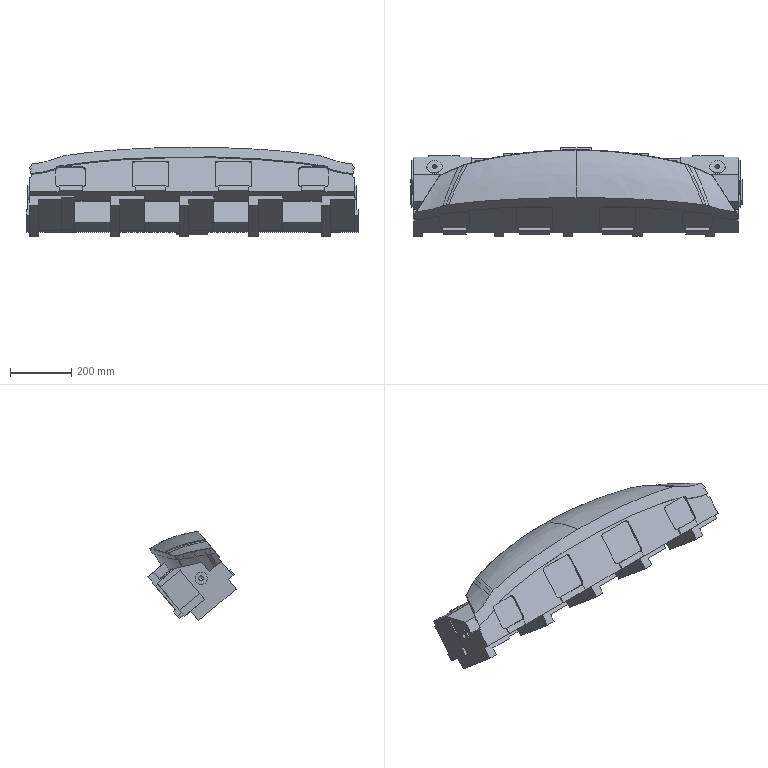Part | NX | features solid 2 | 1 solid | 294 faces | box 1080 x 287.578 x 290.645 mm | volume 34505406 mm3 | plane 175 | spline 77 | cylinder 38 | cone 4 | commonest cylinder face diameters 20 x22 16 x4 60 x4 15 x2 27 x2 40 x2